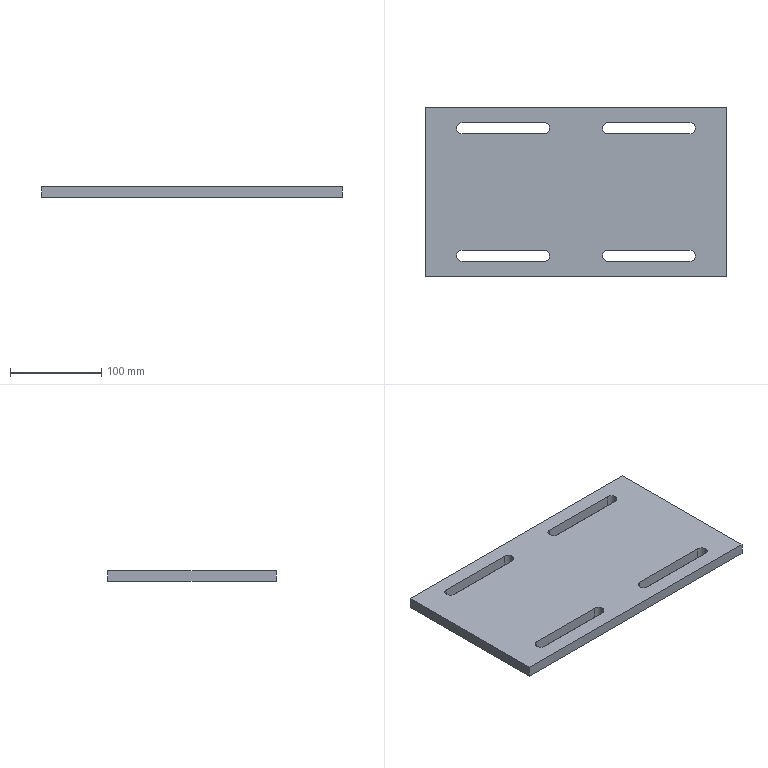Part | SolidWorks | features Chamfer 1, Extrusion 1, HoleWzd 1 | 1 solid | 26 faces | box 330 x 185 x 12 mm | volume 675331 mm3 | plane 14 | cylinder 12 | commonest cylinder face diameters 12 x12
STEP:
#1=CARTESIAN_POINT('',(-29.,70.,-6.));
#2=VERTEX_POINT('',#1);
#3=CARTESIAN_POINT('',(-35.,76.,-6.));
#4=VERTEX_POINT('',#3);
#5=CARTESIAN_POINT('',(-35.,70.,-6.));
#6=DIRECTION('',(0.,0.,1.));
#7=DIRECTION('',(1.,0.,0.));
#8=AXIS2_PLACEMENT_3D('',#5,#6,#7);
#9=CIRCLE('',#8,6.);
#10=EDGE_CURVE('',#2,#4,#9,.T.);
#11=ORIENTED_EDGE('',*,*,#10,.F.);
#12=CARTESIAN_POINT('',(-29.,70.,6.));
#13=VERTEX_POINT('',#12);
#14=CARTESIAN_POINT('',(-29.,70.,6.));
#15=DIRECTION('',(0.,0.,1.));
#16=VECTOR('',#15,1000.);
#17=LINE('',#14,#16);
#18=EDGE_CURVE('',#2,#13,#17,.T.);
#19=ORIENTED_EDGE('',*,*,#18,.T.);
#20=CARTESIAN_POINT('',(-35.,76.,6.));
#21=VERTEX_POINT('',#20);
#22=CARTESIAN_POINT('',(-35.,70.,6.));
#23=DIRECTION('',(0.,0.,1.));
#24=DIRECTION('',(1.,0.,0.));
#25=AXIS2_PLACEMENT_3D('',#22,#23,#24);
#26=CIRCLE('',#25,6.);
#27=EDGE_CURVE('',#13,#21,#26,.T.);
#28=ORIENTED_EDGE('',*,*,#27,.T.);
#29=CARTESIAN_POINT('',(-35.,76.,6.));
#30=DIRECTION('',(0.,0.,1.));
#31=VECTOR('',#30,1000.);
#32=LINE('',#29,#31);
#33=EDGE_CURVE('',#4,#21,#32,.T.);
#34=ORIENTED_EDGE('',*,*,#33,.F.);
#35=EDGE_LOOP('',(#11,#19,#28,#34));
#36=FACE_OUTER_BOUND('',#35,.T.);
#37=CARTESIAN_POINT('',(-35.,70.,6.));
#38=DIRECTION('',(0.,0.,1.));
#39=DIRECTION('',(1.,0.,0.));
#40=AXIS2_PLACEMENT_3D('',#37,#38,#39);
#41=CYLINDRICAL_SURFACE('',#40,6.);
#42=ADVANCED_FACE('',(#36),#41,.F.);
#43=CARTESIAN_POINT('',(131.,70.,-6.));
#44=VERTEX_POINT('',#43);
#45=CARTESIAN_POINT('',(125.,76.,-6.));
#46=VERTEX_POINT('',#45);
#47=CARTESIAN_POINT('',(125.,70.,-6.));
#48=DIRECTION('',(0.,0.,1.));
#49=DIRECTION('',(1.,0.,0.));
#50=AXIS2_PLACEMENT_3D('',#47,#48,#49);
#51=CIRCLE('',#50,6.);
#52=EDGE_CURVE('',#44,#46,#51,.T.);
#53=ORIENTED_EDGE('',*,*,#52,.F.);
#54=CARTESIAN_POINT('',(131.,70.,6.));
#55=VERTEX_POINT('',#54);
#56=CARTESIAN_POINT('',(131.,70.,6.));
#57=DIRECTION('',(0.,0.,1.));
#58=VECTOR('',#57,1000.);
#59=LINE('',#56,#58);
#60=EDGE_CURVE('',#44,#55,#59,.T.);
#61=ORIENTED_EDGE('',*,*,#60,.T.);
#62=CARTESIAN_POINT('',(125.,76.,6.));
#63=VERTEX_POINT('',#62);
#64=CARTESIAN_POINT('',(125.,70.,6.));
#65=DIRECTION('',(0.,0.,1.));
#66=DIRECTION('',(1.,0.,0.));
#67=AXIS2_PLACEMENT_3D('',#64,#65,#66);
#68=CIRCLE('',#67,6.);
#69=EDGE_CURVE('',#55,#63,#68,.T.);
#70=ORIENTED_EDGE('',*,*,#69,.T.);
#71=CARTESIAN_POINT('',(125.,76.,6.));
#72=DIRECTION('',(0.,0.,1.));
#73=VECTOR('',#72,1000.);
#74=LINE('',#71,#73);
#75=EDGE_CURVE('',#46,#63,#74,.T.);
#76=ORIENTED_EDGE('',*,*,#75,.F.);
#77=EDGE_LOOP('',(#53,#61,#70,#76));
#78=FACE_OUTER_BOUND('',#77,.T.);
#79=CARTESIAN_POINT('',(125.,70.,6.));
#80=DIRECTION('',(0.,0.,1.));
#81=DIRECTION('',(1.,0.,0.));
#82=AXIS2_PLACEMENT_3D('',#79,#80,#81);
#83=CYLINDRICAL_SURFACE('',#82,6.);
#84=ADVANCED_FACE('',(#78),#83,.F.);
#85=CARTESIAN_POINT('',(131.,-70.,-6.));
#86=VERTEX_POINT('',#85);
#87=CARTESIAN_POINT('',(125.,-64.,-6.));
#88=VERTEX_POINT('',#87);
#89=CARTESIAN_POINT('',(125.,-70.,-6.));
#90=DIRECTION('',(0.,0.,1.));
#91=DIRECTION('',(1.,0.,0.));
#92=AXIS2_PLACEMENT_3D('',#89,#90,#91);
#93=CIRCLE('',#92,6.);
#94=EDGE_CURVE('',#86,#88,#93,.T.);
#95=ORIENTED_EDGE('',*,*,#94,.F.);
#96=CARTESIAN_POINT('',(131.,-70.,6.));
#97=VERTEX_POINT('',#96);
#98=CARTESIAN_POINT('',(131.,-70.,6.));
#99=DIRECTION('',(0.,0.,1.));
#100=VECTOR('',#99,1000.);
#101=LINE('',#98,#100);
#102=EDGE_CURVE('',#86,#97,#101,.T.);
#103=ORIENTED_EDGE('',*,*,#102,.T.);
#104=CARTESIAN_POINT('',(125.,-64.,6.));
#105=VERTEX_POINT('',#104);
#106=CARTESIAN_POINT('',(125.,-70.,6.));
#107=DIRECTION('',(0.,0.,1.));
#108=DIRECTION('',(1.,0.,0.));
#109=AXIS2_PLACEMENT_3D('',#106,#107,#108);
#110=CIRCLE('',#109,6.);
#111=EDGE_CURVE('',#97,#105,#110,.T.);
#112=ORIENTED_EDGE('',*,*,#111,.T.);
#113=CARTESIAN_POINT('',(125.,-64.,6.));
#114=DIRECTION('',(0.,0.,1.));
#115=VECTOR('',#114,1000.);
#116=LINE('',#113,#115);
#117=EDGE_CURVE('',#88,#105,#116,.T.);
#118=ORIENTED_EDGE('',*,*,#117,.F.);
#119=EDGE_LOOP('',(#95,#103,#112,#118));
#120=FACE_OUTER_BOUND('',#119,.T.);
#121=CARTESIAN_POINT('',(125.,-70.,6.));
#122=DIRECTION('',(0.,0.,1.));
#123=DIRECTION('',(1.,0.,0.));
#124=AXIS2_PLACEMENT_3D('',#121,#122,#123);
#125=CYLINDRICAL_SURFACE('',#124,6.);
#126=ADVANCED_FACE('',(#120),#125,.F.);
#127=CARTESIAN_POINT('',(-29.,-70.,-6.));
#128=VERTEX_POINT('',#127);
#129=CARTESIAN_POINT('',(-35.,-64.,-6.));
#130=VERTEX_POINT('',#129);
#131=CARTESIAN_POINT('',(-35.,-70.,-6.));
#132=DIRECTION('',(0.,0.,1.));
#133=DIRECTION('',(1.,0.,0.));
#134=AXIS2_PLACEMENT_3D('',#131,#132,#133);
#135=CIRCLE('',#134,6.);
#136=EDGE_CURVE('',#128,#130,#135,.T.);
#137=ORIENTED_EDGE('',*,*,#136,.F.);
#138=CARTESIAN_POINT('',(-29.,-70.,6.));
#139=VERTEX_POINT('',#138);
#140=CARTESIAN_POINT('',(-29.,-70.,6.));
#141=DIRECTION('',(0.,0.,1.));
#142=VECTOR('',#141,1000.);
#143=LINE('',#140,#142);
#144=EDGE_CURVE('',#128,#139,#143,.T.);
#145=ORIENTED_EDGE('',*,*,#144,.T.);
#146=CARTESIAN_POINT('',(-35.,-64.,6.));
#147=VERTEX_POINT('',#146);
#148=CARTESIAN_POINT('',(-35.,-70.,6.));
#149=DIRECTION('',(0.,0.,1.));
#150=DIRECTION('',(1.,0.,0.));
#151=AXIS2_PLACEMENT_3D('',#148,#149,#150);
#152=CIRCLE('',#151,6.);
#153=EDGE_CURVE('',#139,#147,#152,.T.);
#154=ORIENTED_EDGE('',*,*,#153,.T.);
#155=CARTESIAN_POINT('',(-35.,-64.,6.));
#156=DIRECTION('',(0.,0.,1.));
#157=VECTOR('',#156,1000.);
#158=LINE('',#155,#157);
#159=EDGE_CURVE('',#130,#147,#158,.T.);
#160=ORIENTED_EDGE('',*,*,#159,.F.);
#161=EDGE_LOOP('',(#137,#145,#154,#160));
#162=FACE_OUTER_BOUND('',#161,.T.);
#163=CARTESIAN_POINT('',(-35.,-70.,6.));
#164=DIRECTION('',(0.,0.,1.));
#165=DIRECTION('',(1.,0.,0.));
#166=AXIS2_PLACEMENT_3D('',#163,#164,#165);
#167=CYLINDRICAL_SURFACE('',#166,6.);
#168=ADVANCED_FACE('',(#162),#167,.F.);
#169=CARTESIAN_POINT('',(-165.,92.5,-6.));
#170=VERTEX_POINT('',#169);
#171=CARTESIAN_POINT('',(-165.,-92.5,-6.));
#172=VERTEX_POINT('',#171);
#173=CARTESIAN_POINT('',(-165.,-92.5,-6.));
#174=DIRECTION('',(0.,-1.,0.));
#175=VECTOR('',#174,1000.);
#176=LINE('',#173,#175);
#177=EDGE_CURVE('',#170,#172,#176,.T.);
#178=ORIENTED_EDGE('',*,*,#177,.T.);
#179=CARTESIAN_POINT('',(-165.,-92.5,6.));
#180=VERTEX_POINT('',#179);
#181=CARTESIAN_POINT('',(-165.,-92.5,6.));
#182=DIRECTION('',(0.,0.,-1.));
#183=VECTOR('',#182,1000.);
#184=LINE('',#181,#183);
#185=EDGE_CURVE('',#180,#172,#184,.T.);
#186=ORIENTED_EDGE('',*,*,#185,.F.);
#187=CARTESIAN_POINT('',(-165.,92.5,6.));
#188=VERTEX_POINT('',#187);
#189=CARTESIAN_POINT('',(-165.,-92.5,6.));
#190=DIRECTION('',(0.,-1.,0.));
#191=VECTOR('',#190,1000.);
#192=LINE('',#189,#191);
#193=EDGE_CURVE('',#188,#180,#192,.T.);
#194=ORIENTED_EDGE('',*,*,#193,.F.);
#195=CARTESIAN_POINT('',(-165.,92.5,6.));
#196=DIRECTION('',(0.,0.,-1.));
#197=VECTOR('',#196,1000.);
#198=LINE('',#195,#197);
#199=EDGE_CURVE('',#188,#170,#198,.T.);
#200=ORIENTED_EDGE('',*,*,#199,.T.);
#201=EDGE_LOOP('',(#178,#186,#194,#200));
#202=FACE_OUTER_BOUND('',#201,.T.);
#203=CARTESIAN_POINT('',(-165.,-92.5,6.));
#204=DIRECTION('',(1.,0.,0.));
#205=DIRECTION('',(0.,0.,-1.));
#206=AXIS2_PLACEMENT_3D('',#203,#204,#205);
#207=PLANE('',#206);
#208=ADVANCED_FACE('',(#202),#207,.F.);
#209=CARTESIAN_POINT('',(165.,-92.5,-6.));
#210=VERTEX_POINT('',#209);
#211=CARTESIAN_POINT('',(165.,-92.5,-6.));
#212=DIRECTION('',(1.,0.,0.));
#213=VECTOR('',#212,1000.);
#214=LINE('',#211,#213);
#215=EDGE_CURVE('',#172,#210,#214,.T.);
#216=ORIENTED_EDGE('',*,*,#215,.T.);
#217=CARTESIAN_POINT('',(165.,-92.5,6.));
#218=VERTEX_POINT('',#217);
#219=CARTESIAN_POINT('',(165.,-92.5,6.));
#220=DIRECTION('',(0.,0.,-1.));
#221=VECTOR('',#220,1000.);
#222=LINE('',#219,#221);
#223=EDGE_CURVE('',#218,#210,#222,.T.);
#224=ORIENTED_EDGE('',*,*,#223,.F.);
#225=CARTESIAN_POINT('',(165.,-92.5,6.));
#226=DIRECTION('',(1.,0.,0.));
#227=VECTOR('',#226,1000.);
#228=LINE('',#225,#227);
#229=EDGE_CURVE('',#180,#218,#228,.T.);
#230=ORIENTED_EDGE('',*,*,#229,.F.);
#231=ORIENTED_EDGE('',*,*,#185,.T.);
#232=EDGE_LOOP('',(#216,#224,#230,#231));
#233=FACE_OUTER_BOUND('',#232,.T.);
#234=CARTESIAN_POINT('',(165.,-92.5,6.));
#235=DIRECTION('',(0.,1.,0.));
#236=DIRECTION('',(-1.,0.,0.));
#237=AXIS2_PLACEMENT_3D('',#234,#235,#236);
#238=PLANE('',#237);
#239=ADVANCED_FACE('',(#233),#238,.F.);
#240=CARTESIAN_POINT('',(165.,92.5,-6.));
#241=VERTEX_POINT('',#240);
#242=CARTESIAN_POINT('',(165.,-92.5,-6.));
#243=DIRECTION('',(0.,1.,0.));
#244=VECTOR('',#243,1000.);
#245=LINE('',#242,#244);
#246=EDGE_CURVE('',#210,#241,#245,.T.);
#247=ORIENTED_EDGE('',*,*,#246,.T.);
#248=CARTESIAN_POINT('',(165.,92.5,6.));
#249=VERTEX_POINT('',#248);
#250=CARTESIAN_POINT('',(165.,92.5,6.));
#251=DIRECTION('',(0.,0.,-1.));
#252=VECTOR('',#251,1000.);
#253=LINE('',#250,#252);
#254=EDGE_CURVE('',#249,#241,#253,.T.);
#255=ORIENTED_EDGE('',*,*,#254,.F.);
#256=CARTESIAN_POINT('',(165.,-92.5,6.));
#257=DIRECTION('',(0.,1.,0.));
#258=VECTOR('',#257,1000.);
#259=LINE('',#256,#258);
#260=EDGE_CURVE('',#218,#249,#259,.T.);
#261=ORIENTED_EDGE('',*,*,#260,.F.);
#262=ORIENTED_EDGE('',*,*,#223,.T.);
#263=EDGE_LOOP('',(#247,#255,#261,#262));
#264=FACE_OUTER_BOUND('',#263,.T.);
#265=CARTESIAN_POINT('',(165.,-92.5,6.));
#266=DIRECTION('',(-1.,0.,0.));
#267=DIRECTION('',(0.,0.,1.));
#268=AXIS2_PLACEMENT_3D('',#265,#266,#267);
#269=PLANE('',#268);
#270=ADVANCED_FACE('',(#264),#269,.F.);
#271=CARTESIAN_POINT('',(165.,92.5,-6.));
#272=DIRECTION('',(-1.,0.,0.));
#273=VECTOR('',#272,1000.);
#274=LINE('',#271,#273);
#275=EDGE_CURVE('',#241,#170,#274,.T.);
#276=ORIENTED_EDGE('',*,*,#275,.T.);
#277=ORIENTED_EDGE('',*,*,#199,.F.);
#278=CARTESIAN_POINT('',(165.,92.5,6.));
#279=DIRECTION('',(-1.,0.,0.));
#280=VECTOR('',#279,1000.);
#281=LINE('',#278,#280);
#282=EDGE_CURVE('',#249,#188,#281,.T.);
#283=ORIENTED_EDGE('',*,*,#282,.F.);
#284=ORIENTED_EDGE('',*,*,#254,.T.);
#285=EDGE_LOOP('',(#276,#277,#283,#284));
#286=FACE_OUTER_BOUND('',#285,.T.);
#287=CARTESIAN_POINT('',(165.,92.5,6.));
#288=DIRECTION('',(0.,-1.,0.));
#289=DIRECTION('',(1.,0.,0.));
#290=AXIS2_PLACEMENT_3D('',#287,#288,#289);
#291=PLANE('',#290);
#292=ADVANCED_FACE('',(#286),#291,.F.);
#293=CARTESIAN_POINT('',(-125.,64.,6.));
#294=VERTEX_POINT('',#293);
#295=CARTESIAN_POINT('',(-35.,64.,6.));
#296=VERTEX_POINT('',#295);
#297=CARTESIAN_POINT('',(-125.,64.,6.));
#298=DIRECTION('',(1.,0.,0.));
#299=VECTOR('',#298,1000.);
#300=LINE('',#297,#299);
#301=EDGE_CURVE('',#294,#296,#300,.T.);
#302=ORIENTED_EDGE('',*,*,#301,.F.);
#303=CARTESIAN_POINT('',(-125.,76.,6.));
#304=VERTEX_POINT('',#303);
#305=CARTESIAN_POINT('',(-125.,70.,6.));
#306=DIRECTION('',(0.,0.,1.));
#307=DIRECTION('',(1.,0.,0.));
#308=AXIS2_PLACEMENT_3D('',#305,#306,#307);
#309=CIRCLE('',#308,6.);
#310=EDGE_CURVE('',#304,#294,#309,.T.);
#311=ORIENTED_EDGE('',*,*,#310,.F.);
#312=CARTESIAN_POINT('',(-125.,76.,6.));
#313=DIRECTION('',(1.,0.,0.));
#314=VECTOR('',#313,1000.);
#315=LINE('',#312,#314);
#316=EDGE_CURVE('',#304,#21,#315,.T.);
#317=ORIENTED_EDGE('',*,*,#316,.T.);
#318=ORIENTED_EDGE('',*,*,#27,.F.);
#319=CARTESIAN_POINT('',(-35.,70.,6.));
#320=DIRECTION('',(0.,0.,1.));
#321=DIRECTION('',(1.,0.,0.));
#322=AXIS2_PLACEMENT_3D('',#319,#320,#321);
#323=CIRCLE('',#322,6.);
#324=EDGE_CURVE('',#296,#13,#323,.T.);
#325=ORIENTED_EDGE('',*,*,#324,.F.);
#326=EDGE_LOOP('',(#302,#311,#317,#318,#325));
#327=FACE_BOUND('',#326,.T.);
#328=CARTESIAN_POINT('',(125.,64.,6.));
#329=VERTEX_POINT('',#328);
#330=CARTESIAN_POINT('',(125.,70.,6.));
#331=DIRECTION('',(0.,0.,1.));
#332=DIRECTION('',(1.,0.,0.));
#333=AXIS2_PLACEMENT_3D('',#330,#331,#332);
#334=CIRCLE('',#333,6.);
#335=EDGE_CURVE('',#329,#55,#334,.T.);
#336=ORIENTED_EDGE('',*,*,#335,.F.);
#337=CARTESIAN_POINT('',(35.,64.,6.));
#338=VERTEX_POINT('',#337);
#339=CARTESIAN_POINT('',(35.,64.,6.));
#340=DIRECTION('',(1.,0.,0.));
#341=VECTOR('',#340,1000.);
#342=LINE('',#339,#341);
#343=EDGE_CURVE('',#338,#329,#342,.T.);
#344=ORIENTED_EDGE('',*,*,#343,.F.);
#345=CARTESIAN_POINT('',(35.,76.,6.));
#346=VERTEX_POINT('',#345);
#347=CARTESIAN_POINT('',(35.,70.,6.));
#348=DIRECTION('',(0.,0.,1.));
#349=DIRECTION('',(1.,0.,0.));
#350=AXIS2_PLACEMENT_3D('',#347,#348,#349);
#351=CIRCLE('',#350,6.);
#352=EDGE_CURVE('',#346,#338,#351,.T.);
#353=ORIENTED_EDGE('',*,*,#352,.F.);
#354=CARTESIAN_POINT('',(35.,76.,6.));
#355=DIRECTION('',(1.,0.,0.));
#356=VECTOR('',#355,1000.);
#357=LINE('',#354,#356);
#358=EDGE_CURVE('',#346,#63,#357,.T.);
#359=ORIENTED_EDGE('',*,*,#358,.T.);
#360=ORIENTED_EDGE('',*,*,#69,.F.);
#361=EDGE_LOOP('',(#336,#344,#353,#359,#360));
#362=FACE_BOUND('',#361,.T.);
#363=CARTESIAN_POINT('',(35.,-76.,6.));
#364=VERTEX_POINT('',#363);
#365=CARTESIAN_POINT('',(125.,-76.,6.));
#366=VERTEX_POINT('',#365);
#367=CARTESIAN_POINT('',(35.,-76.,6.));
#368=DIRECTION('',(1.,0.,0.));
#369=VECTOR('',#368,1000.);
#370=LINE('',#367,#369);
#371=EDGE_CURVE('',#364,#366,#370,.T.);
#372=ORIENTED_EDGE('',*,*,#371,.F.);
#373=CARTESIAN_POINT('',(35.,-64.,6.));
#374=VERTEX_POINT('',#373);
#375=CARTESIAN_POINT('',(35.,-70.,6.));
#376=DIRECTION('',(0.,0.,1.));
#377=DIRECTION('',(1.,0.,0.));
#378=AXIS2_PLACEMENT_3D('',#375,#376,#377);
#379=CIRCLE('',#378,6.);
#380=EDGE_CURVE('',#374,#364,#379,.T.);
#381=ORIENTED_EDGE('',*,*,#380,.F.);
#382=CARTESIAN_POINT('',(35.,-64.,6.));
#383=DIRECTION('',(1.,0.,0.));
#384=VECTOR('',#383,1000.);
#385=LINE('',#382,#384);
#386=EDGE_CURVE('',#374,#105,#385,.T.);
#387=ORIENTED_EDGE('',*,*,#386,.T.);
#388=ORIENTED_EDGE('',*,*,#111,.F.);
#389=CARTESIAN_POINT('',(125.,-70.,6.));
#390=DIRECTION('',(0.,0.,1.));
#391=DIRECTION('',(1.,0.,0.));
#392=AXIS2_PLACEMENT_3D('',#389,#390,#391);
#393=CIRCLE('',#392,6.);
#394=EDGE_CURVE('',#366,#97,#393,.T.);
#395=ORIENTED_EDGE('',*,*,#394,.F.);
#396=EDGE_LOOP('',(#372,#381,#387,#388,#395));
#397=FACE_BOUND('',#396,.T.);
#398=CARTESIAN_POINT('',(-35.,-76.,6.));
#399=VERTEX_POINT('',#398);
#400=CARTESIAN_POINT('',(-35.,-70.,6.));
#401=DIRECTION('',(0.,0.,1.));
#402=DIRECTION('',(1.,0.,0.));
#403=AXIS2_PLACEMENT_3D('',#400,#401,#402);
#404=CIRCLE('',#403,6.);
#405=EDGE_CURVE('',#399,#139,#404,.T.);
#406=ORIENTED_EDGE('',*,*,#405,.F.);
#407=CARTESIAN_POINT('',(-125.,-76.,6.));
#408=VERTEX_POINT('',#407);
#409=CARTESIAN_POINT('',(-125.,-76.,6.));
#410=DIRECTION('',(1.,0.,0.));
#411=VECTOR('',#410,1000.);
#412=LINE('',#409,#411);
#413=EDGE_CURVE('',#408,#399,#412,.T.);
#414=ORIENTED_EDGE('',*,*,#413,.F.);
#415=CARTESIAN_POINT('',(-125.,-64.,6.));
#416=VERTEX_POINT('',#415);
#417=CARTESIAN_POINT('',(-125.,-70.,6.));
#418=DIRECTION('',(0.,0.,1.));
#419=DIRECTION('',(1.,0.,0.));
#420=AXIS2_PLACEMENT_3D('',#417,#418,#419);
#421=CIRCLE('',#420,6.);
#422=EDGE_CURVE('',#416,#408,#421,.T.);
#423=ORIENTED_EDGE('',*,*,#422,.F.);
#424=CARTESIAN_POINT('',(-125.,-64.,6.));
#425=DIRECTION('',(1.,0.,0.));
#426=VECTOR('',#425,1000.);
#427=LINE('',#424,#426);
#428=EDGE_CURVE('',#416,#147,#427,.T.);
#429=ORIENTED_EDGE('',*,*,#428,.T.);
#430=ORIENTED_EDGE('',*,*,#153,.F.);
#431=EDGE_LOOP('',(#406,#414,#423,#429,#430));
#432=FACE_BOUND('',#431,.T.);
#433=ORIENTED_EDGE('',*,*,#193,.T.);
#434=ORIENTED_EDGE('',*,*,#229,.T.);
#435=ORIENTED_EDGE('',*,*,#260,.T.);
#436=ORIENTED_EDGE('',*,*,#282,.T.);
#437=EDGE_LOOP('',(#433,#434,#435,#436));
#438=FACE_OUTER_BOUND('',#437,.T.);
#439=CARTESIAN_POINT('',(0.,0.,6.));
#440=DIRECTION('',(0.,0.,1.));
#441=DIRECTION('',(1.,0.,0.));
#442=AXIS2_PLACEMENT_3D('',#439,#440,#441);
#443=PLANE('',#442);
#444=ADVANCED_FACE('',(#327,#362,#397,#432,#438),#443,.T.);
#445=CARTESIAN_POINT('',(-35.,64.,-6.));
#446=VERTEX_POINT('',#445);
#447=CARTESIAN_POINT('',(-35.,70.,-6.));
#448=DIRECTION('',(0.,0.,1.));
#449=DIRECTION('',(1.,0.,0.));
#450=AXIS2_PLACEMENT_3D('',#447,#448,#449);
#451=CIRCLE('',#450,6.);
#452=EDGE_CURVE('',#446,#2,#451,.T.);
#453=ORIENTED_EDGE('',*,*,#452,.T.);
#454=ORIENTED_EDGE('',*,*,#10,.T.);
#455=CARTESIAN_POINT('',(-125.,76.,-6.));
#456=VERTEX_POINT('',#455);
#457=CARTESIAN_POINT('',(0.,76.,-6.));
#458=DIRECTION('',(-1.,0.,0.));
#459=VECTOR('',#458,1000.);
#460=LINE('',#457,#459);
#461=EDGE_CURVE('',#4,#456,#460,.T.);
#462=ORIENTED_EDGE('',*,*,#461,.T.);
#463=CARTESIAN_POINT('',(-125.,64.,-6.));
#464=VERTEX_POINT('',#463);
#465=CARTESIAN_POINT('',(-125.,70.,-6.));
#466=DIRECTION('',(0.,0.,1.));
#467=DIRECTION('',(1.,0.,0.));
#468=AXIS2_PLACEMENT_3D('',#465,#466,#467);
#469=CIRCLE('',#468,6.);
#470=EDGE_CURVE('',#456,#464,#469,.T.);
#471=ORIENTED_EDGE('',*,*,#470,.T.);
#472=CARTESIAN_POINT('',(0.,64.,-6.));
#473=DIRECTION('',(1.,0.,0.));
#474=VECTOR('',#473,1000.);
#475=LINE('',#472,#474);
#476=EDGE_CURVE('',#464,#446,#475,.T.);
#477=ORIENTED_EDGE('',*,*,#476,.T.);
#478=EDGE_LOOP('',(#453,#454,#462,#471,#477));
#479=FACE_BOUND('',#478,.T.);
#480=CARTESIAN_POINT('',(125.,64.,-6.));
#481=VERTEX_POINT('',#480);
#482=CARTESIAN_POINT('',(125.,70.,-6.));
#483=DIRECTION('',(0.,0.,1.));
#484=DIRECTION('',(1.,0.,0.));
#485=AXIS2_PLACEMENT_3D('',#482,#483,#484);
#486=CIRCLE('',#485,6.);
#487=EDGE_CURVE('',#481,#44,#486,.T.);
#488=ORIENTED_EDGE('',*,*,#487,.T.);
#489=ORIENTED_EDGE('',*,*,#52,.T.);
#490=CARTESIAN_POINT('',(35.,76.,-6.));
#491=VERTEX_POINT('',#490);
#492=CARTESIAN_POINT('',(0.,76.,-6.));
#493=DIRECTION('',(-1.,0.,0.));
#494=VECTOR('',#493,1000.);
#495=LINE('',#492,#494);
#496=EDGE_CURVE('',#46,#491,#495,.T.);
#497=ORIENTED_EDGE('',*,*,#496,.T.);
#498=CARTESIAN_POINT('',(35.,64.,-6.));
#499=VERTEX_POINT('',#498);
#500=CARTESIAN_POINT('',(35.,70.,-6.));
#501=DIRECTION('',(0.,0.,1.));
#502=DIRECTION('',(1.,0.,0.));
#503=AXIS2_PLACEMENT_3D('',#500,#501,#502);
#504=CIRCLE('',#503,6.);
#505=EDGE_CURVE('',#491,#499,#504,.T.);
#506=ORIENTED_EDGE('',*,*,#505,.T.);
#507=CARTESIAN_POINT('',(0.,64.,-6.));
#508=DIRECTION('',(1.,0.,0.));
#509=VECTOR('',#508,1000.);
#510=LINE('',#507,#509);
#511=EDGE_CURVE('',#499,#481,#510,.T.);
#512=ORIENTED_EDGE('',*,*,#511,.T.);
#513=EDGE_LOOP('',(#488,#489,#497,#506,#512));
#514=FACE_BOUND('',#513,.T.);
#515=CARTESIAN_POINT('',(125.,-76.,-6.));
#516=VERTEX_POINT('',#515);
#517=CARTESIAN_POINT('',(125.,-70.,-6.));
#518=DIRECTION('',(0.,0.,1.));
#519=DIRECTION('',(1.,0.,0.));
#520=AXIS2_PLACEMENT_3D('',#517,#518,#519);
#521=CIRCLE('',#520,6.);
#522=EDGE_CURVE('',#516,#86,#521,.T.);
#523=ORIENTED_EDGE('',*,*,#522,.T.);
#524=ORIENTED_EDGE('',*,*,#94,.T.);
#525=CARTESIAN_POINT('',(35.,-64.,-6.));
#526=VERTEX_POINT('',#525);
#527=CARTESIAN_POINT('',(0.,-64.,-6.));
#528=DIRECTION('',(-1.,0.,0.));
#529=VECTOR('',#528,1000.);
#530=LINE('',#527,#529);
#531=EDGE_CURVE('',#88,#526,#530,.T.);
#532=ORIENTED_EDGE('',*,*,#531,.T.);
#533=CARTESIAN_POINT('',(35.,-76.,-6.));
#534=VERTEX_POINT('',#533);
#535=CARTESIAN_POINT('',(35.,-70.,-6.));
#536=DIRECTION('',(0.,0.,1.));
#537=DIRECTION('',(1.,0.,0.));
#538=AXIS2_PLACEMENT_3D('',#535,#536,#537);
#539=CIRCLE('',#538,6.);
#540=EDGE_CURVE('',#526,#534,#539,.T.);
#541=ORIENTED_EDGE('',*,*,#540,.T.);
#542=CARTESIAN_POINT('',(0.,-76.,-6.));
#543=DIRECTION('',(1.,0.,0.));
#544=VECTOR('',#543,1000.);
#545=LINE('',#542,#544);
#546=EDGE_CURVE('',#534,#516,#545,.T.);
#547=ORIENTED_EDGE('',*,*,#546,.T.);
#548=EDGE_LOOP('',(#523,#524,#532,#541,#547));
#549=FACE_BOUND('',#548,.T.);
#550=CARTESIAN_POINT('',(-35.,-76.,-6.));
#551=VERTEX_POINT('',#550);
#552=CARTESIAN_POINT('',(-35.,-70.,-6.));
#553=DIRECTION('',(0.,0.,1.));
#554=DIRECTION('',(1.,0.,0.));
#555=AXIS2_PLACEMENT_3D('',#552,#553,#554);
#556=CIRCLE('',#555,6.);
#557=EDGE_CURVE('',#551,#128,#556,.T.);
#558=ORIENTED_EDGE('',*,*,#557,.T.);
#559=ORIENTED_EDGE('',*,*,#136,.T.);
#560=CARTESIAN_POINT('',(-125.,-64.,-6.));
#561=VERTEX_POINT('',#560);
#562=CARTESIAN_POINT('',(0.,-64.,-6.));
#563=DIRECTION('',(-1.,0.,0.));
#564=VECTOR('',#563,1000.);
#565=LINE('',#562,#564);
#566=EDGE_CURVE('',#130,#561,#565,.T.);
#567=ORIENTED_EDGE('',*,*,#566,.T.);
#568=CARTESIAN_POINT('',(-125.,-76.,-6.));
#569=VERTEX_POINT('',#568);
#570=CARTESIAN_POINT('',(-125.,-70.,-6.));
#571=DIRECTION('',(0.,0.,1.));
#572=DIRECTION('',(1.,0.,0.));
#573=AXIS2_PLACEMENT_3D('',#570,#571,#572);
#574=CIRCLE('',#573,6.);
#575=EDGE_CURVE('',#561,#569,#574,.T.);
#576=ORIENTED_EDGE('',*,*,#575,.T.);
#577=CARTESIAN_POINT('',(0.,-76.,-6.));
#578=DIRECTION('',(1.,0.,0.));
#579=VECTOR('',#578,1000.);
#580=LINE('',#577,#579);
#581=EDGE_CURVE('',#569,#551,#580,.T.);
#582=ORIENTED_EDGE('',*,*,#581,.T.);
#583=EDGE_LOOP('',(#558,#559,#567,#576,#582));
#584=FACE_BOUND('',#583,.T.);
#585=ORIENTED_EDGE('',*,*,#177,.F.);
#586=ORIENTED_EDGE('',*,*,#275,.F.);
#587=ORIENTED_EDGE('',*,*,#246,.F.);
#588=ORIENTED_EDGE('',*,*,#215,.F.);
#589=EDGE_LOOP('',(#585,#586,#587,#588));
#590=FACE_OUTER_BOUND('',#589,.T.);
#591=CARTESIAN_POINT('',(0.,0.,-6.));
#592=DIRECTION('',(0.,0.,1.));
#593=DIRECTION('',(1.,0.,0.));
#594=AXIS2_PLACEMENT_3D('',#591,#592,#593);
#595=PLANE('',#594);
#596=ADVANCED_FACE('',(#479,#514,#549,#584,#590),#595,.F.);
#597=ORIENTED_EDGE('',*,*,#144,.F.);
#598=ORIENTED_EDGE('',*,*,#557,.F.);
#599=CARTESIAN_POINT('',(-35.,-76.,6.));
#600=DIRECTION('',(0.,0.,-1.));
#601=VECTOR('',#600,1000.);
#602=LINE('',#599,#601);
#603=EDGE_CURVE('',#399,#551,#602,.T.);
#604=ORIENTED_EDGE('',*,*,#603,.F.);
#605=ORIENTED_EDGE('',*,*,#405,.T.);
#606=EDGE_LOOP('',(#597,#598,#604,#605));
#607=FACE_OUTER_BOUND('',#606,.T.);
#608=CARTESIAN_POINT('',(-35.,-70.,6.));
#609=DIRECTION('',(0.,0.,1.));
#610=DIRECTION('',(1.,0.,0.));
#611=AXIS2_PLACEMENT_3D('',#608,#609,#610);
#612=CYLINDRICAL_SURFACE('',#611,6.);
#613=ADVANCED_FACE('',(#607),#612,.F.);
#614=CARTESIAN_POINT('',(-125.,-64.,6.));
#615=DIRECTION('',(0.,0.,-1.));
#616=VECTOR('',#615,1000.);
#617=LINE('',#614,#616);
#618=EDGE_CURVE('',#416,#561,#617,.T.);
#619=ORIENTED_EDGE('',*,*,#618,.F.);
#620=ORIENTED_EDGE('',*,*,#422,.T.);
#621=CARTESIAN_POINT('',(-125.,-76.,6.));
#622=DIRECTION('',(0.,0.,1.));
#623=VECTOR('',#622,1000.);
#624=LINE('',#621,#623);
#625=EDGE_CURVE('',#569,#408,#624,.T.);
#626=ORIENTED_EDGE('',*,*,#625,.F.);
#627=ORIENTED_EDGE('',*,*,#575,.F.);
#628=EDGE_LOOP('',(#619,#620,#626,#627));
#629=FACE_OUTER_BOUND('',#628,.T.);
#630=CARTESIAN_POINT('',(-125.,-70.,6.));
#631=DIRECTION('',(0.,0.,1.));
#632=DIRECTION('',(1.,0.,0.));
#633=AXIS2_PLACEMENT_3D('',#630,#631,#632);
#634=CYLINDRICAL_SURFACE('',#633,6.);
#635=ADVANCED_FACE('',(#629),#634,.F.);
#636=ORIENTED_EDGE('',*,*,#159,.T.);
#637=ORIENTED_EDGE('',*,*,#428,.F.);
#638=ORIENTED_EDGE('',*,*,#618,.T.);
#639=ORIENTED_EDGE('',*,*,#566,.F.);
#640=EDGE_LOOP('',(#636,#637,#638,#639));
#641=FACE_OUTER_BOUND('',#640,.T.);
#642=CARTESIAN_POINT('',(-125.,-64.,6.));
#643=DIRECTION('',(0.,1.,0.));
#644=DIRECTION('',(0.,0.,1.));
#645=AXIS2_PLACEMENT_3D('',#642,#643,#644);
#646=PLANE('',#645);
#647=ADVANCED_FACE('',(#641),#646,.F.);
#648=ORIENTED_EDGE('',*,*,#625,.T.);
#649=ORIENTED_EDGE('',*,*,#413,.T.);
#650=ORIENTED_EDGE('',*,*,#603,.T.);
#651=ORIENTED_EDGE('',*,*,#581,.F.);
#652=EDGE_LOOP('',(#648,#649,#650,#651));
#653=FACE_OUTER_BOUND('',#652,.T.);
#654=CARTESIAN_POINT('',(-125.,-76.,6.));
#655=DIRECTION('',(0.,-1.,0.));
#656=DIRECTION('',(0.,0.,-1.));
#657=AXIS2_PLACEMENT_3D('',#654,#655,#656);
#658=PLANE('',#657);
#659=ADVANCED_FACE('',(#653),#658,.F.);
#660=ORIENTED_EDGE('',*,*,#102,.F.);
#661=ORIENTED_EDGE('',*,*,#522,.F.);
#662=CARTESIAN_POINT('',(125.,-76.,6.));
#663=DIRECTION('',(0.,0.,-1.));
#664=VECTOR('',#663,1000.);
#665=LINE('',#662,#664);
#666=EDGE_CURVE('',#366,#516,#665,.T.);
#667=ORIENTED_EDGE('',*,*,#666,.F.);
#668=ORIENTED_EDGE('',*,*,#394,.T.);
#669=EDGE_LOOP('',(#660,#661,#667,#668));
#670=FACE_OUTER_BOUND('',#669,.T.);
#671=CARTESIAN_POINT('',(125.,-70.,6.));
#672=DIRECTION('',(0.,0.,1.));
#673=DIRECTION('',(1.,0.,0.));
#674=AXIS2_PLACEMENT_3D('',#671,#672,#673);
#675=CYLINDRICAL_SURFACE('',#674,6.);
#676=ADVANCED_FACE('',(#670),#675,.F.);
#677=CARTESIAN_POINT('',(35.,-64.,6.));
#678=DIRECTION('',(0.,0.,-1.));
#679=VECTOR('',#678,1000.);
#680=LINE('',#677,#679);
#681=EDGE_CURVE('',#374,#526,#680,.T.);
#682=ORIENTED_EDGE('',*,*,#681,.F.);
#683=ORIENTED_EDGE('',*,*,#380,.T.);
#684=CARTESIAN_POINT('',(35.,-76.,6.));
#685=DIRECTION('',(0.,0.,1.));
#686=VECTOR('',#685,1000.);
#687=LINE('',#684,#686);
#688=EDGE_CURVE('',#534,#364,#687,.T.);
#689=ORIENTED_EDGE('',*,*,#688,.F.);
#690=ORIENTED_EDGE('',*,*,#540,.F.);
#691=EDGE_LOOP('',(#682,#683,#689,#690));
#692=FACE_OUTER_BOUND('',#691,.T.);
#693=CARTESIAN_POINT('',(35.,-70.,6.));
#694=DIRECTION('',(0.,0.,1.));
#695=DIRECTION('',(1.,0.,0.));
#696=AXIS2_PLACEMENT_3D('',#693,#694,#695);
#697=CYLINDRICAL_SURFACE('',#696,6.);
#698=ADVANCED_FACE('',(#692),#697,.F.);
#699=ORIENTED_EDGE('',*,*,#117,.T.);
#700=ORIENTED_EDGE('',*,*,#386,.F.);
#701=ORIENTED_EDGE('',*,*,#681,.T.);
#702=ORIENTED_EDGE('',*,*,#531,.F.);
#703=EDGE_LOOP('',(#699,#700,#701,#702));
#704=FACE_OUTER_BOUND('',#703,.T.);
#705=CARTESIAN_POINT('',(35.,-64.,6.));
#706=DIRECTION('',(0.,1.,0.));
#707=DIRECTION('',(0.,0.,1.));
#708=AXIS2_PLACEMENT_3D('',#705,#706,#707);
#709=PLANE('',#708);
#710=ADVANCED_FACE('',(#704),#709,.F.);
#711=ORIENTED_EDGE('',*,*,#688,.T.);
#712=ORIENTED_EDGE('',*,*,#371,.T.);
#713=ORIENTED_EDGE('',*,*,#666,.T.);
#714=ORIENTED_EDGE('',*,*,#546,.F.);
#715=EDGE_LOOP('',(#711,#712,#713,#714));
#716=FACE_OUTER_BOUND('',#715,.T.);
#717=CARTESIAN_POINT('',(35.,-76.,6.));
#718=DIRECTION('',(0.,-1.,0.));
#719=DIRECTION('',(0.,0.,-1.));
#720=AXIS2_PLACEMENT_3D('',#717,#718,#719);
#721=PLANE('',#720);
#722=ADVANCED_FACE('',(#716),#721,.F.);
#723=ORIENTED_EDGE('',*,*,#60,.F.);
#724=ORIENTED_EDGE('',*,*,#487,.F.);
#725=CARTESIAN_POINT('',(125.,64.,6.));
#726=DIRECTION('',(0.,0.,-1.));
#727=VECTOR('',#726,1000.);
#728=LINE('',#725,#727);
#729=EDGE_CURVE('',#329,#481,#728,.T.);
#730=ORIENTED_EDGE('',*,*,#729,.F.);
#731=ORIENTED_EDGE('',*,*,#335,.T.);
#732=EDGE_LOOP('',(#723,#724,#730,#731));
#733=FACE_OUTER_BOUND('',#732,.T.);
#734=CARTESIAN_POINT('',(125.,70.,6.));
#735=DIRECTION('',(0.,0.,1.));
#736=DIRECTION('',(1.,0.,0.));
#737=AXIS2_PLACEMENT_3D('',#734,#735,#736);
#738=CYLINDRICAL_SURFACE('',#737,6.);
#739=ADVANCED_FACE('',(#733),#738,.F.);
#740=CARTESIAN_POINT('',(35.,76.,6.));
#741=DIRECTION('',(0.,0.,-1.));
#742=VECTOR('',#741,1000.);
#743=LINE('',#740,#742);
#744=EDGE_CURVE('',#346,#491,#743,.T.);
#745=ORIENTED_EDGE('',*,*,#744,.F.);
#746=ORIENTED_EDGE('',*,*,#352,.T.);
#747=CARTESIAN_POINT('',(35.,64.,6.));
#748=DIRECTION('',(0.,0.,1.));
#749=VECTOR('',#748,1000.);
#750=LINE('',#747,#749);
#751=EDGE_CURVE('',#499,#338,#750,.T.);
#752=ORIENTED_EDGE('',*,*,#751,.F.);
#753=ORIENTED_EDGE('',*,*,#505,.F.);
#754=EDGE_LOOP('',(#745,#746,#752,#753));
#755=FACE_OUTER_BOUND('',#754,.T.);
#756=CARTESIAN_POINT('',(35.,70.,6.));
#757=DIRECTION('',(0.,0.,1.));
#758=DIRECTION('',(1.,0.,0.));
#759=AXIS2_PLACEMENT_3D('',#756,#757,#758);
#760=CYLINDRICAL_SURFACE('',#759,6.);
#761=ADVANCED_FACE('',(#755),#760,.F.);
#762=ORIENTED_EDGE('',*,*,#75,.T.);
#763=ORIENTED_EDGE('',*,*,#358,.F.);
#764=ORIENTED_EDGE('',*,*,#744,.T.);
#765=ORIENTED_EDGE('',*,*,#496,.F.);
#766=EDGE_LOOP('',(#762,#763,#764,#765));
#767=FACE_OUTER_BOUND('',#766,.T.);
#768=CARTESIAN_POINT('',(35.,76.,6.));
#769=DIRECTION('',(0.,1.,0.));
#770=DIRECTION('',(0.,0.,1.));
#771=AXIS2_PLACEMENT_3D('',#768,#769,#770);
#772=PLANE('',#771);
#773=ADVANCED_FACE('',(#767),#772,.F.);
#774=ORIENTED_EDGE('',*,*,#751,.T.);
#775=ORIENTED_EDGE('',*,*,#343,.T.);
#776=ORIENTED_EDGE('',*,*,#729,.T.);
#777=ORIENTED_EDGE('',*,*,#511,.F.);
#778=EDGE_LOOP('',(#774,#775,#776,#777));
#779=FACE_OUTER_BOUND('',#778,.T.);
#780=CARTESIAN_POINT('',(35.,64.,6.));
#781=DIRECTION('',(0.,-1.,0.));
#782=DIRECTION('',(0.,0.,-1.));
#783=AXIS2_PLACEMENT_3D('',#780,#781,#782);
#784=PLANE('',#783);
#785=ADVANCED_FACE('',(#779),#784,.F.);
#786=ORIENTED_EDGE('',*,*,#18,.F.);
#787=ORIENTED_EDGE('',*,*,#452,.F.);
#788=CARTESIAN_POINT('',(-35.,64.,6.));
#789=DIRECTION('',(0.,0.,-1.));
#790=VECTOR('',#789,1000.);
#791=LINE('',#788,#790);
#792=EDGE_CURVE('',#296,#446,#791,.T.);
#793=ORIENTED_EDGE('',*,*,#792,.F.);
#794=ORIENTED_EDGE('',*,*,#324,.T.);
#795=EDGE_LOOP('',(#786,#787,#793,#794));
#796=FACE_OUTER_BOUND('',#795,.T.);
#797=CARTESIAN_POINT('',(-35.,70.,6.));
#798=DIRECTION('',(0.,0.,1.));
#799=DIRECTION('',(1.,0.,0.));
#800=AXIS2_PLACEMENT_3D('',#797,#798,#799);
#801=CYLINDRICAL_SURFACE('',#800,6.);
#802=ADVANCED_FACE('',(#796),#801,.F.);
#803=CARTESIAN_POINT('',(-125.,76.,6.));
#804=DIRECTION('',(0.,0.,-1.));
#805=VECTOR('',#804,1000.);
#806=LINE('',#803,#805);
#807=EDGE_CURVE('',#304,#456,#806,.T.);
#808=ORIENTED_EDGE('',*,*,#807,.F.);
#809=ORIENTED_EDGE('',*,*,#310,.T.);
#810=CARTESIAN_POINT('',(-125.,64.,6.));
#811=DIRECTION('',(0.,0.,1.));
#812=VECTOR('',#811,1000.);
#813=LINE('',#810,#812);
#814=EDGE_CURVE('',#464,#294,#813,.T.);
#815=ORIENTED_EDGE('',*,*,#814,.F.);
#816=ORIENTED_EDGE('',*,*,#470,.F.);
#817=EDGE_LOOP('',(#808,#809,#815,#816));
#818=FACE_OUTER_BOUND('',#817,.T.);
#819=CARTESIAN_POINT('',(-125.,70.,6.));
#820=DIRECTION('',(0.,0.,1.));
#821=DIRECTION('',(1.,0.,0.));
#822=AXIS2_PLACEMENT_3D('',#819,#820,#821);
#823=CYLINDRICAL_SURFACE('',#822,6.);
#824=ADVANCED_FACE('',(#818),#823,.F.);
#825=ORIENTED_EDGE('',*,*,#33,.T.);
#826=ORIENTED_EDGE('',*,*,#316,.F.);
#827=ORIENTED_EDGE('',*,*,#807,.T.);
#828=ORIENTED_EDGE('',*,*,#461,.F.);
#829=EDGE_LOOP('',(#825,#826,#827,#828));
#830=FACE_OUTER_BOUND('',#829,.T.);
#831=CARTESIAN_POINT('',(-125.,76.,6.));
#832=DIRECTION('',(0.,1.,0.));
#833=DIRECTION('',(0.,0.,1.));
#834=AXIS2_PLACEMENT_3D('',#831,#832,#833);
#835=PLANE('',#834);
#836=ADVANCED_FACE('',(#830),#835,.F.);
#837=ORIENTED_EDGE('',*,*,#814,.T.);
#838=ORIENTED_EDGE('',*,*,#301,.T.);
#839=ORIENTED_EDGE('',*,*,#792,.T.);
#840=ORIENTED_EDGE('',*,*,#476,.F.);
#841=EDGE_LOOP('',(#837,#838,#839,#840));
#842=FACE_OUTER_BOUND('',#841,.T.);
#843=CARTESIAN_POINT('',(-125.,64.,6.));
#844=DIRECTION('',(0.,-1.,0.));
#845=DIRECTION('',(0.,0.,-1.));
#846=AXIS2_PLACEMENT_3D('',#843,#844,#845);
#847=PLANE('',#846);
#848=ADVANCED_FACE('',(#842),#847,.F.);
#849=CLOSED_SHELL('',(#42,#84,#126,#168,#208,#239,#270,#292,#444,#596,#613,#635,#647,#659,#676,#698,#710,#722,#739,#761,#773,#785,#802,#824,#836,#848));
#850=MANIFOLD_SOLID_BREP('',#849);
#851=CARTESIAN_POINT('',(0.,0.,0.));
#852=DIRECTION('',(0.,0.,1.));
#853=DIRECTION('',(1.,0.,0.));
#854=AXIS2_PLACEMENT_3D('',#851,#852,#853);
#855=(LENGTH_UNIT()NAMED_UNIT(*)SI_UNIT(.MILLI.,.METRE.));
#856=UNCERTAINTY_MEASURE_WITH_UNIT(LENGTH_MEASURE(0.00001),#855,'','');
#857=(NAMED_UNIT(*)PLANE_ANGLE_UNIT()SI_UNIT($,.RADIAN.));
#858=(NAMED_UNIT(*)SI_UNIT($,.STERADIAN.)SOLID_ANGLE_UNIT());
#859=(GEOMETRIC_REPRESENTATION_CONTEXT(3)GLOBAL_UNCERTAINTY_ASSIGNED_CONTEXT((#856))GLOBAL_UNIT_ASSIGNED_CONTEXT((#855,#857,#858))REPRESENTATION_CONTEXT('',''));
#860=ADVANCED_BREP_SHAPE_REPRESENTATION('',(#850,#854),#859);